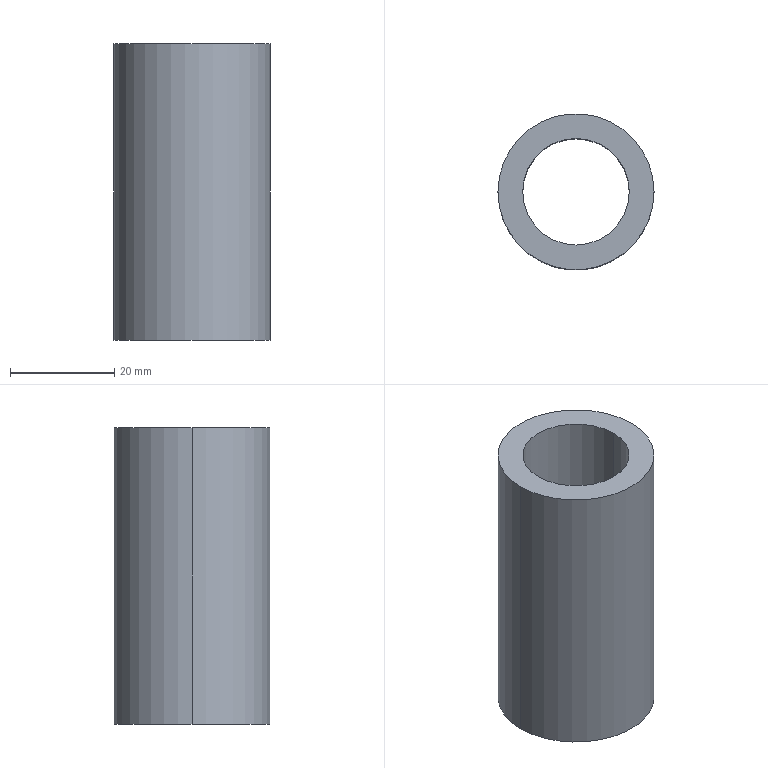Part | SolidWorks | features Chamfer 1, Extrusion 1 | 1 solid | 6 faces | box 30 x 30 x 57 mm | volume 21477 mm3 | cylinder 4 | plane 2 | commonest cylinder face diameters 20.5 x2 30 x2
STEP:
#1=CARTESIAN_POINT('',(-10.25,0.,28.5));
#2=VERTEX_POINT('',#1);
#3=CARTESIAN_POINT('',(10.25,0.,28.5));
#4=VERTEX_POINT('',#3);
#5=CARTESIAN_POINT('',(0.,0.,28.5));
#6=DIRECTION('',(0.,0.,1.));
#7=DIRECTION('',(1.,0.,0.));
#8=AXIS2_PLACEMENT_3D('',#5,#6,#7);
#9=CIRCLE('',#8,10.25);
#10=EDGE_CURVE('',#2,#4,#9,.T.);
#11=ORIENTED_EDGE('',*,*,#10,.T.);
#12=CARTESIAN_POINT('',(10.25,0.,-28.5));
#13=VERTEX_POINT('',#12);
#14=CARTESIAN_POINT('',(10.25,0.,28.5));
#15=DIRECTION('',(0.,0.,-1.));
#16=VECTOR('',#15,1000.);
#17=LINE('',#14,#16);
#18=EDGE_CURVE('',#4,#13,#17,.T.);
#19=ORIENTED_EDGE('',*,*,#18,.T.);
#20=CARTESIAN_POINT('',(-10.25,0.,-28.5));
#21=VERTEX_POINT('',#20);
#22=CARTESIAN_POINT('',(0.,0.,-28.5));
#23=DIRECTION('',(0.,0.,1.));
#24=DIRECTION('',(1.,0.,0.));
#25=AXIS2_PLACEMENT_3D('',#22,#23,#24);
#26=CIRCLE('',#25,10.25);
#27=EDGE_CURVE('',#21,#13,#26,.T.);
#28=ORIENTED_EDGE('',*,*,#27,.F.);
#29=CARTESIAN_POINT('',(-10.25,0.,28.5));
#30=DIRECTION('',(0.,0.,-1.));
#31=VECTOR('',#30,1000.);
#32=LINE('',#29,#31);
#33=EDGE_CURVE('',#2,#21,#32,.T.);
#34=ORIENTED_EDGE('',*,*,#33,.F.);
#35=EDGE_LOOP('',(#11,#19,#28,#34));
#36=FACE_OUTER_BOUND('',#35,.T.);
#37=CARTESIAN_POINT('',(0.,0.,28.5));
#38=DIRECTION('',(0.,0.,-1.));
#39=DIRECTION('',(-1.,0.,0.));
#40=AXIS2_PLACEMENT_3D('',#37,#38,#39);
#41=CYLINDRICAL_SURFACE('',#40,10.25);
#42=ADVANCED_FACE('',(#36),#41,.F.);
#43=CARTESIAN_POINT('',(15.,0.,28.5));
#44=VERTEX_POINT('',#43);
#45=CARTESIAN_POINT('',(-15.,0.,28.5));
#46=VERTEX_POINT('',#45);
#47=CARTESIAN_POINT('',(0.,0.,28.5));
#48=DIRECTION('',(0.,0.,1.));
#49=DIRECTION('',(1.,0.,0.));
#50=AXIS2_PLACEMENT_3D('',#47,#48,#49);
#51=CIRCLE('',#50,15.);
#52=EDGE_CURVE('',#44,#46,#51,.T.);
#53=ORIENTED_EDGE('',*,*,#52,.F.);
#54=CARTESIAN_POINT('',(15.,0.,-28.5));
#55=VERTEX_POINT('',#54);
#56=CARTESIAN_POINT('',(15.,0.,28.5));
#57=DIRECTION('',(0.,0.,-1.));
#58=VECTOR('',#57,1000.);
#59=LINE('',#56,#58);
#60=EDGE_CURVE('',#44,#55,#59,.T.);
#61=ORIENTED_EDGE('',*,*,#60,.T.);
#62=CARTESIAN_POINT('',(-15.,0.,-28.5));
#63=VERTEX_POINT('',#62);
#64=CARTESIAN_POINT('',(0.,0.,-28.5));
#65=DIRECTION('',(0.,0.,1.));
#66=DIRECTION('',(1.,0.,0.));
#67=AXIS2_PLACEMENT_3D('',#64,#65,#66);
#68=CIRCLE('',#67,15.);
#69=EDGE_CURVE('',#55,#63,#68,.T.);
#70=ORIENTED_EDGE('',*,*,#69,.T.);
#71=CARTESIAN_POINT('',(-15.,0.,28.5));
#72=DIRECTION('',(0.,0.,-1.));
#73=VECTOR('',#72,1000.);
#74=LINE('',#71,#73);
#75=EDGE_CURVE('',#46,#63,#74,.T.);
#76=ORIENTED_EDGE('',*,*,#75,.F.);
#77=EDGE_LOOP('',(#53,#61,#70,#76));
#78=FACE_OUTER_BOUND('',#77,.T.);
#79=CARTESIAN_POINT('',(0.,0.,28.5));
#80=DIRECTION('',(0.,0.,-1.));
#81=DIRECTION('',(-1.,0.,0.));
#82=AXIS2_PLACEMENT_3D('',#79,#80,#81);
#83=CYLINDRICAL_SURFACE('',#82,15.);
#84=ADVANCED_FACE('',(#78),#83,.T.);
#85=CARTESIAN_POINT('',(0.,0.,28.5));
#86=DIRECTION('',(0.,0.,1.));
#87=DIRECTION('',(1.,0.,0.));
#88=AXIS2_PLACEMENT_3D('',#85,#86,#87);
#89=CIRCLE('',#88,15.);
#90=EDGE_CURVE('',#46,#44,#89,.T.);
#91=ORIENTED_EDGE('',*,*,#90,.T.);
#92=ORIENTED_EDGE('',*,*,#52,.T.);
#93=EDGE_LOOP('',(#91,#92));
#94=FACE_OUTER_BOUND('',#93,.T.);
#95=ORIENTED_EDGE('',*,*,#10,.F.);
#96=CARTESIAN_POINT('',(0.,0.,28.5));
#97=DIRECTION('',(0.,0.,1.));
#98=DIRECTION('',(1.,0.,0.));
#99=AXIS2_PLACEMENT_3D('',#96,#97,#98);
#100=CIRCLE('',#99,10.25);
#101=EDGE_CURVE('',#4,#2,#100,.T.);
#102=ORIENTED_EDGE('',*,*,#101,.F.);
#103=EDGE_LOOP('',(#95,#102));
#104=FACE_BOUND('',#103,.T.);
#105=CARTESIAN_POINT('',(0.,0.,28.5));
#106=DIRECTION('',(0.,0.,1.));
#107=DIRECTION('',(1.,0.,0.));
#108=AXIS2_PLACEMENT_3D('',#105,#106,#107);
#109=PLANE('',#108);
#110=ADVANCED_FACE('',(#94,#104),#109,.T.);
#111=CARTESIAN_POINT('',(0.,0.,-28.5));
#112=DIRECTION('',(0.,0.,1.));
#113=DIRECTION('',(1.,0.,0.));
#114=AXIS2_PLACEMENT_3D('',#111,#112,#113);
#115=CIRCLE('',#114,15.);
#116=EDGE_CURVE('',#63,#55,#115,.T.);
#117=ORIENTED_EDGE('',*,*,#116,.F.);
#118=ORIENTED_EDGE('',*,*,#69,.F.);
#119=EDGE_LOOP('',(#117,#118));
#120=FACE_OUTER_BOUND('',#119,.T.);
#121=ORIENTED_EDGE('',*,*,#27,.T.);
#122=CARTESIAN_POINT('',(0.,0.,-28.5));
#123=DIRECTION('',(0.,0.,1.));
#124=DIRECTION('',(1.,0.,0.));
#125=AXIS2_PLACEMENT_3D('',#122,#123,#124);
#126=CIRCLE('',#125,10.25);
#127=EDGE_CURVE('',#13,#21,#126,.T.);
#128=ORIENTED_EDGE('',*,*,#127,.T.);
#129=EDGE_LOOP('',(#121,#128));
#130=FACE_BOUND('',#129,.T.);
#131=CARTESIAN_POINT('',(0.,0.,-28.5));
#132=DIRECTION('',(0.,0.,1.));
#133=DIRECTION('',(1.,0.,0.));
#134=AXIS2_PLACEMENT_3D('',#131,#132,#133);
#135=PLANE('',#134);
#136=ADVANCED_FACE('',(#120,#130),#135,.F.);
#137=ORIENTED_EDGE('',*,*,#60,.F.);
#138=ORIENTED_EDGE('',*,*,#90,.F.);
#139=ORIENTED_EDGE('',*,*,#75,.T.);
#140=ORIENTED_EDGE('',*,*,#116,.T.);
#141=EDGE_LOOP('',(#137,#138,#139,#140));
#142=FACE_OUTER_BOUND('',#141,.T.);
#143=CARTESIAN_POINT('',(0.,0.,28.5));
#144=DIRECTION('',(0.,0.,-1.));
#145=DIRECTION('',(-1.,0.,0.));
#146=AXIS2_PLACEMENT_3D('',#143,#144,#145);
#147=CYLINDRICAL_SURFACE('',#146,15.);
#148=ADVANCED_FACE('',(#142),#147,.T.);
#149=ORIENTED_EDGE('',*,*,#18,.F.);
#150=ORIENTED_EDGE('',*,*,#101,.T.);
#151=ORIENTED_EDGE('',*,*,#33,.T.);
#152=ORIENTED_EDGE('',*,*,#127,.F.);
#153=EDGE_LOOP('',(#149,#150,#151,#152));
#154=FACE_OUTER_BOUND('',#153,.T.);
#155=CARTESIAN_POINT('',(0.,0.,28.5));
#156=DIRECTION('',(0.,0.,-1.));
#157=DIRECTION('',(-1.,0.,0.));
#158=AXIS2_PLACEMENT_3D('',#155,#156,#157);
#159=CYLINDRICAL_SURFACE('',#158,10.25);
#160=ADVANCED_FACE('',(#154),#159,.F.);
#161=CLOSED_SHELL('',(#42,#84,#110,#136,#148,#160));
#162=MANIFOLD_SOLID_BREP('',#161);
#163=CARTESIAN_POINT('',(0.,0.,0.));
#164=DIRECTION('',(0.,0.,1.));
#165=DIRECTION('',(1.,0.,0.));
#166=AXIS2_PLACEMENT_3D('',#163,#164,#165);
#167=(LENGTH_UNIT()NAMED_UNIT(*)SI_UNIT(.MILLI.,.METRE.));
#168=UNCERTAINTY_MEASURE_WITH_UNIT(LENGTH_MEASURE(0.00001),#167,'','');
#169=(NAMED_UNIT(*)PLANE_ANGLE_UNIT()SI_UNIT($,.RADIAN.));
#170=(NAMED_UNIT(*)SI_UNIT($,.STERADIAN.)SOLID_ANGLE_UNIT());
#171=(GEOMETRIC_REPRESENTATION_CONTEXT(3)GLOBAL_UNCERTAINTY_ASSIGNED_CONTEXT((#168))GLOBAL_UNIT_ASSIGNED_CONTEXT((#167,#169,#170))REPRESENTATION_CONTEXT('',''));
#172=ADVANCED_BREP_SHAPE_REPRESENTATION('',(#162,#166),#171);